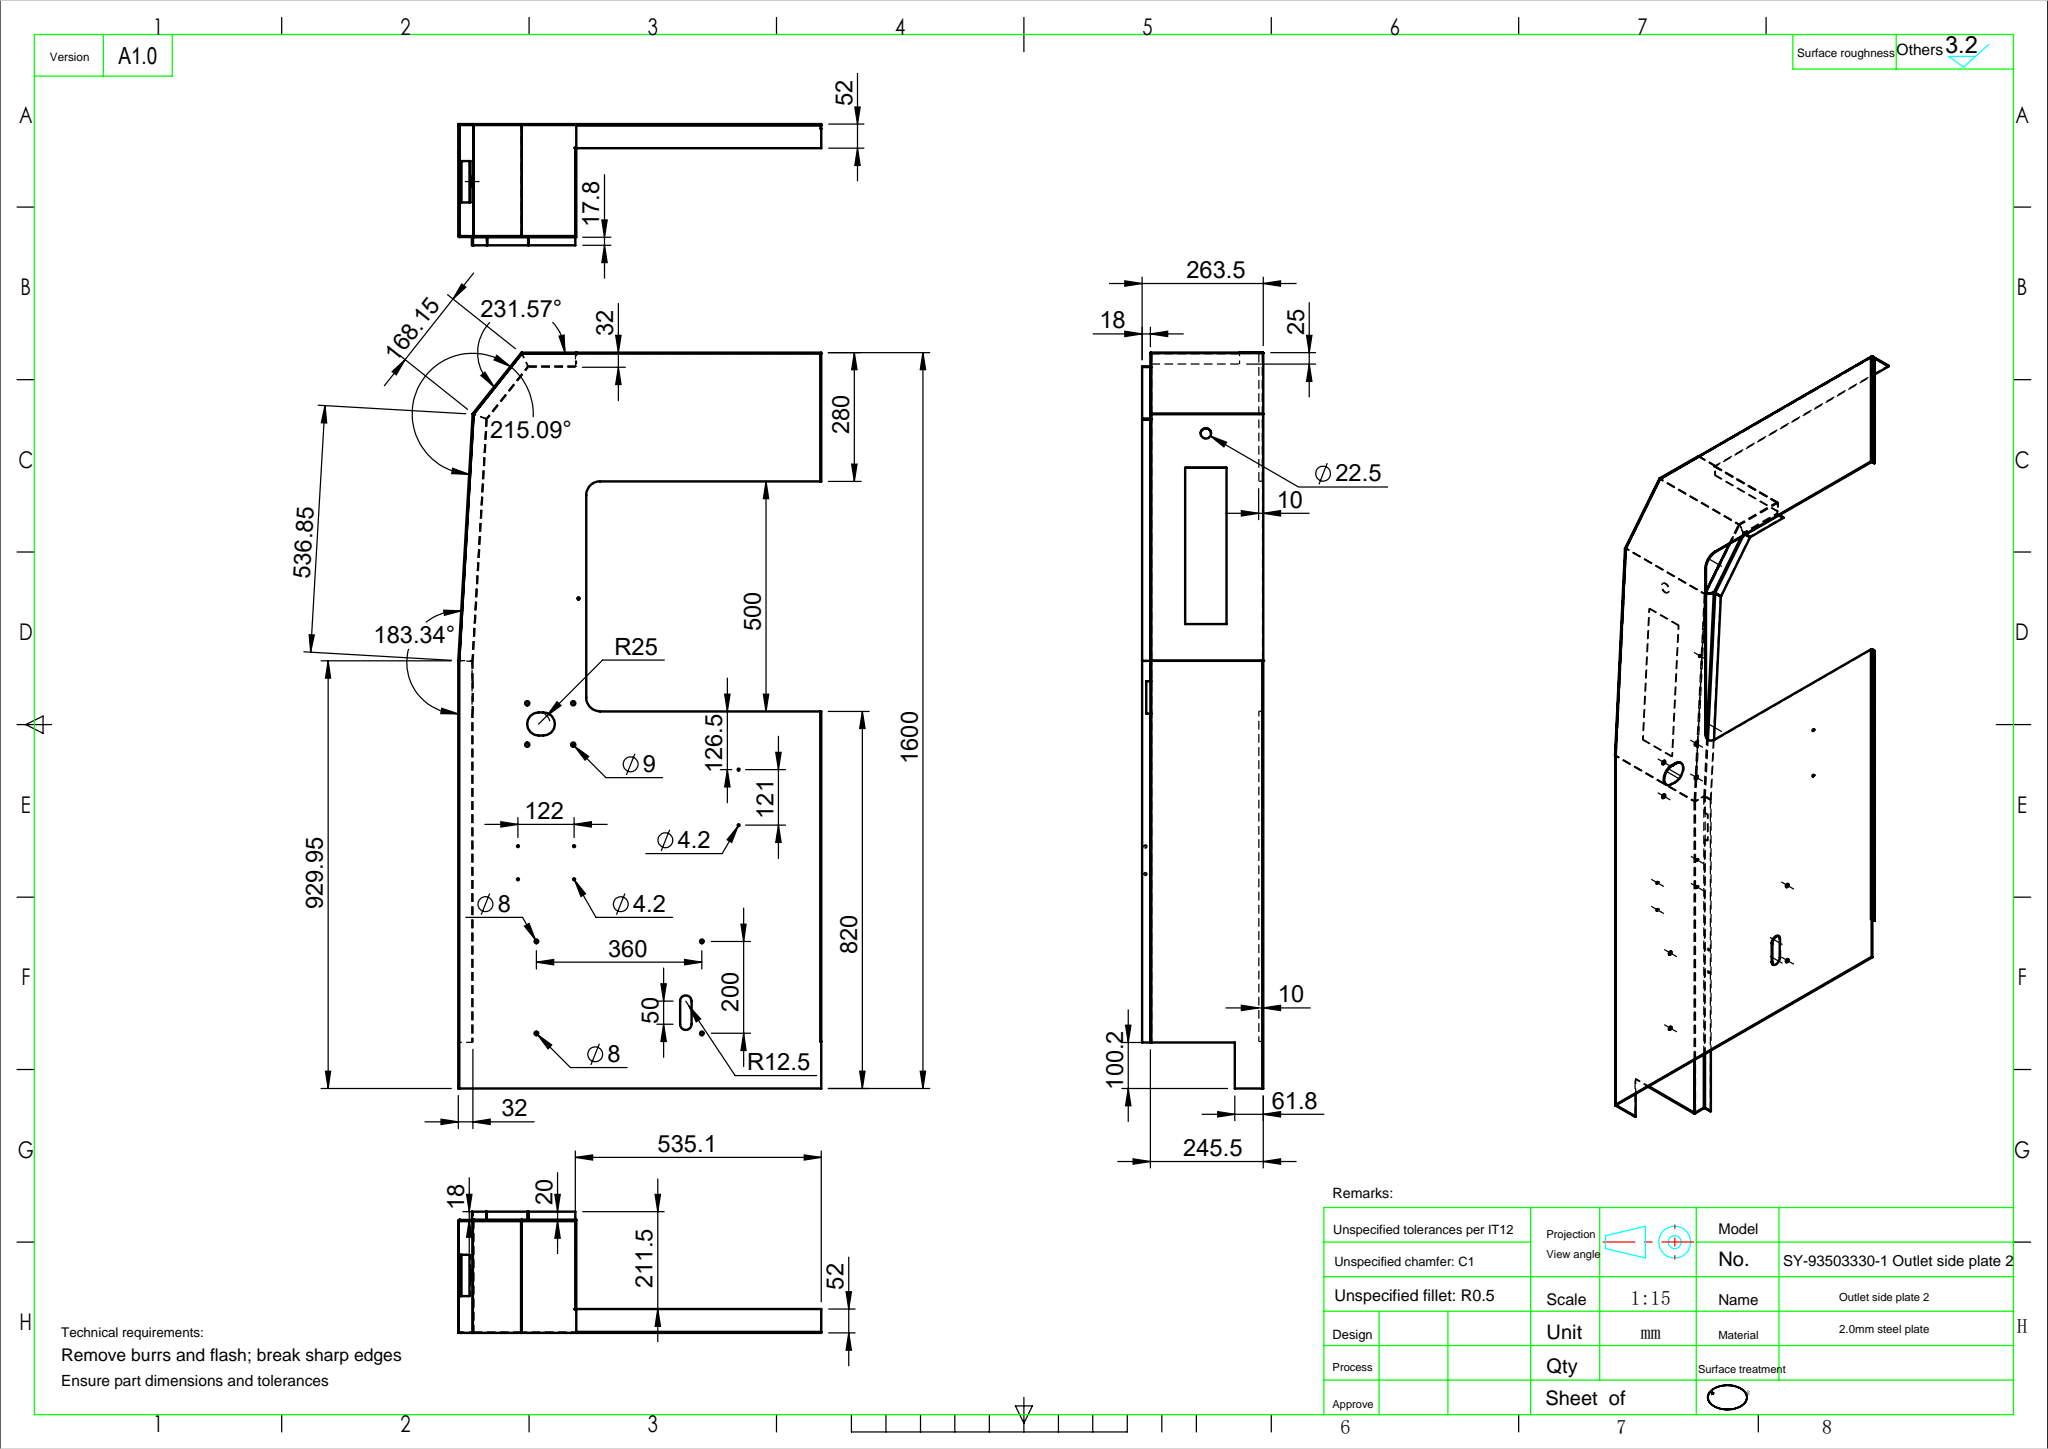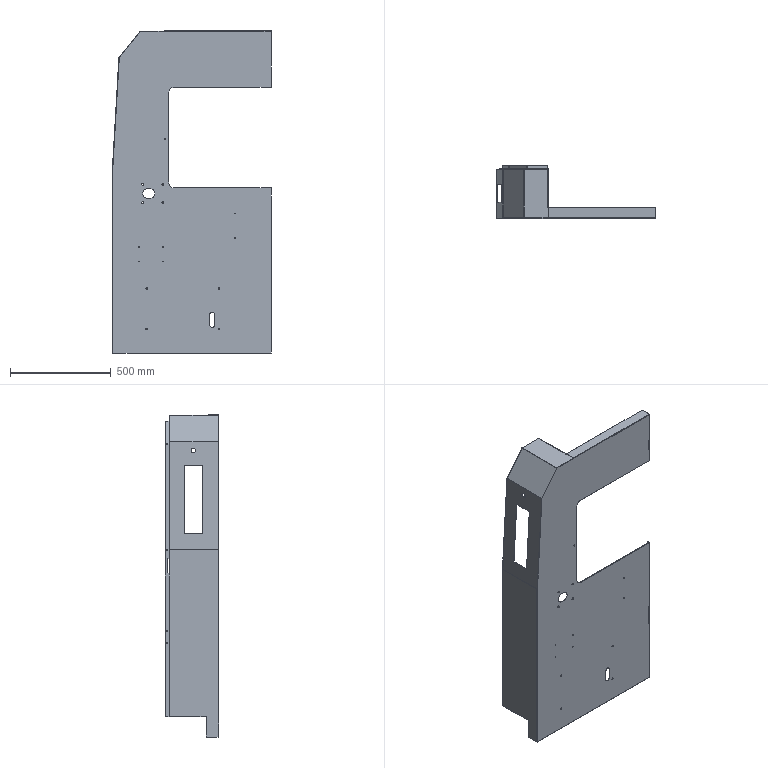Part | SolidWorks | features ICE 17, EdgeFlange 8, Cut 5, FlatPattern 2, HoleWzd 2, SMBaseFlange 2, SheetMetal 2, 3DProfileFeature 1, DelFace 1 | 2 solids | 220 faces | box 789.9 x 263.5 x 1600 mm | volume 2950026 mm3 | plane 137 | cylinder 79 | spline 4 | commonest cylinder face diameters 0.4 x16 4.2 x16 4.4 x15 8 x8 9 x8 1 x5